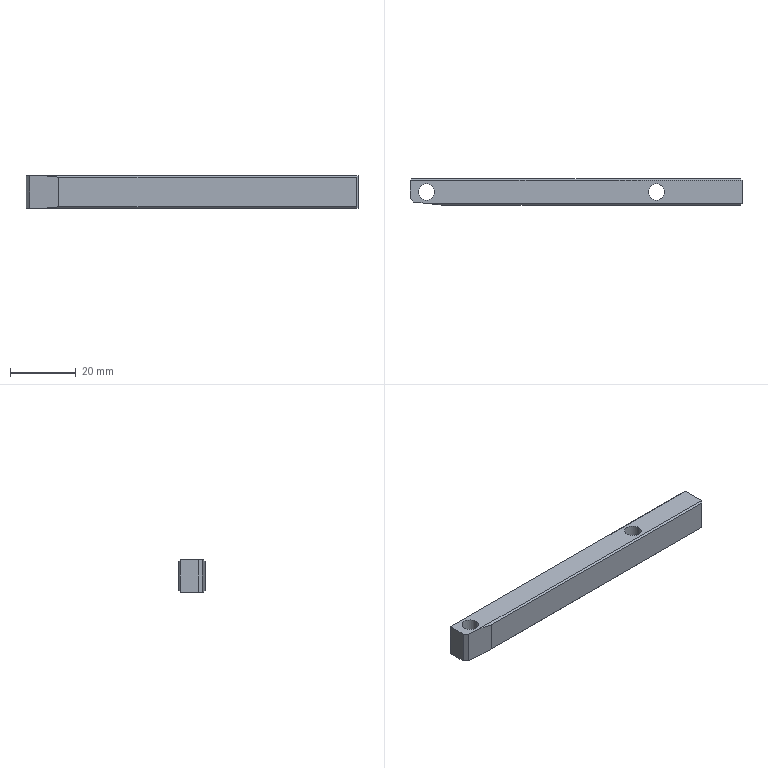Part | SolidWorks | features Chamfer 2, Extrusion 1, HoleWzd 1, ICE 1 | 1 solid | 21 faces | box 101 x 8 x 10 mm | volume 7248 mm3 | plane 15 | cylinder 6 | commonest cylinder face diameters 5 x4 4.2 x2
STEP:
#1=CARTESIAN_POINT('',(27.,0.,2.1));
#2=VERTEX_POINT('',#1);
#3=CARTESIAN_POINT('',(27.,0.,-2.1));
#4=VERTEX_POINT('',#3);
#5=CARTESIAN_POINT('',(27.,0.,2.1));
#6=CARTESIAN_POINT('',(27.,-0.1478,2.1));
#7=CARTESIAN_POINT('',(26.987,-0.2944,2.084));
#8=CARTESIAN_POINT('',(26.937,-0.5774,2.024));
#9=CARTESIAN_POINT('',(26.899,-0.7152,1.979));
#10=CARTESIAN_POINT('',(26.808,-0.9708,1.867));
#11=CARTESIAN_POINT('',(26.753,-1.091,1.799));
#12=CARTESIAN_POINT('',(26.632,-1.311,1.646));
#13=CARTESIAN_POINT('',(26.567,-1.411,1.561));
#14=CARTESIAN_POINT('',(26.431,-1.592,1.376));
#15=CARTESIAN_POINT('',(26.359,-1.674,1.274));
#16=CARTESIAN_POINT('',(26.22,-1.817,1.06));
#17=CARTESIAN_POINT('',(26.151,-1.879,0.9468));
#18=CARTESIAN_POINT('',(26.024,-1.983,0.703));
#19=CARTESIAN_POINT('',(25.966,-2.026,0.5719));
#20=CARTESIAN_POINT('',(25.882,-2.084,0.2961));
#21=CARTESIAN_POINT('',(25.857,-2.1,0.1485));
#22=CARTESIAN_POINT('',(25.856,-2.1,-0.1436));
#23=CARTESIAN_POINT('',(25.881,-2.084,-0.2919));
#24=CARTESIAN_POINT('',(25.965,-2.026,-0.5686));
#25=CARTESIAN_POINT('',(26.023,-1.984,-0.6998));
#26=CARTESIAN_POINT('',(26.212,-1.829,-1.065));
#27=CARTESIAN_POINT('',(26.361,-1.684,-1.281));
#28=CARTESIAN_POINT('',(26.566,-1.412,-1.559));
#29=CARTESIAN_POINT('',(26.632,-1.311,-1.646));
#30=CARTESIAN_POINT('',(26.753,-1.091,-1.799));
#31=CARTESIAN_POINT('',(26.807,-0.9728,-1.866));
#32=CARTESIAN_POINT('',(26.945,-0.5883,-2.035));
#33=CARTESIAN_POINT('',(27.,-0.2971,-2.1));
#34=CARTESIAN_POINT('',(27.,0.,-2.1));
#35=B_SPLINE_CURVE_WITH_KNOTS('',3,(#5,#6,#7,#8,#9,#10,#11,#12,#13,#14,#15,#16,#17,#18,#19,#20,#21,#22,#23,#24,#25,#26,#27,#28,#29,#30,#31,#32,#33,#34),.UNSPECIFIED.,.F.,.F.,(4,2,2,2,2,2,2,2,2,2,2,2,2,2,4),(0.007025,0.007463,0.007902,0.00834,0.008778,0.009216,0.009655,0.01009,0.01053,0.01097,0.01141,0.01228,0.01272,0.01316,0.01404),.UNSPECIFIED.);
#36=EDGE_CURVE('',#2,#4,#35,.T.);
#37=ORIENTED_EDGE('',*,*,#36,.F.);
#38=CARTESIAN_POINT('',(50.5,0.,2.1));
#39=VERTEX_POINT('',#38);
#40=CARTESIAN_POINT('',(50.5,0.,2.1));
#41=DIRECTION('',(1.,0.,0.));
#42=VECTOR('',#41,1000.);
#43=LINE('',#40,#42);
#44=EDGE_CURVE('',#2,#39,#43,.T.);
#45=ORIENTED_EDGE('',*,*,#44,.T.);
#46=CARTESIAN_POINT('',(50.5,0.,-2.1));
#47=VERTEX_POINT('',#46);
#48=CARTESIAN_POINT('',(50.5,0.,0.));
#49=DIRECTION('',(1.,0.,0.));
#50=DIRECTION('',(0.,0.,-1.));
#51=AXIS2_PLACEMENT_3D('',#48,#49,#50);
#52=CIRCLE('',#51,2.1);
#53=EDGE_CURVE('',#39,#47,#52,.T.);
#54=ORIENTED_EDGE('',*,*,#53,.T.);
#55=CARTESIAN_POINT('',(50.5,0.,-2.1));
#56=DIRECTION('',(1.,0.,0.));
#57=VECTOR('',#56,1000.);
#58=LINE('',#55,#57);
#59=EDGE_CURVE('',#4,#47,#58,.T.);
#60=ORIENTED_EDGE('',*,*,#59,.F.);
#61=EDGE_LOOP('',(#37,#45,#54,#60));
#62=FACE_OUTER_BOUND('',#61,.T.);
#63=CARTESIAN_POINT('',(50.5,0.,0.));
#64=DIRECTION('',(1.,0.,0.));
#65=DIRECTION('',(0.,0.,-1.));
#66=AXIS2_PLACEMENT_3D('',#63,#64,#65);
#67=CYLINDRICAL_SURFACE('',#66,2.1);
#68=ADVANCED_FACE('',(#62),#67,.F.);
#69=CARTESIAN_POINT('',(22.,0.,-5.));
#70=VERTEX_POINT('',#69);
#71=CARTESIAN_POINT('',(27.,0.,-5.));
#72=VERTEX_POINT('',#71);
#73=CARTESIAN_POINT('',(24.5,0.,-5.));
#74=DIRECTION('',(0.,0.,1.));
#75=DIRECTION('',(1.,0.,0.));
#76=AXIS2_PLACEMENT_3D('',#73,#74,#75);
#77=CIRCLE('',#76,2.5);
#78=EDGE_CURVE('',#70,#72,#77,.T.);
#79=ORIENTED_EDGE('',*,*,#78,.F.);
#80=CARTESIAN_POINT('',(22.,0.,5.));
#81=VERTEX_POINT('',#80);
#82=CARTESIAN_POINT('',(22.,0.,-5.));
#83=DIRECTION('',(0.,0.,1.));
#84=VECTOR('',#83,1000.);
#85=LINE('',#82,#84);
#86=EDGE_CURVE('',#70,#81,#85,.T.);
#87=ORIENTED_EDGE('',*,*,#86,.T.);
#88=CARTESIAN_POINT('',(27.,0.,5.));
#89=VERTEX_POINT('',#88);
#90=CARTESIAN_POINT('',(24.5,0.,5.));
#91=DIRECTION('',(0.,0.,1.));
#92=DIRECTION('',(1.,0.,0.));
#93=AXIS2_PLACEMENT_3D('',#90,#91,#92);
#94=CIRCLE('',#93,2.5);
#95=EDGE_CURVE('',#81,#89,#94,.T.);
#96=ORIENTED_EDGE('',*,*,#95,.T.);
#97=CARTESIAN_POINT('',(27.,0.,-5.));
#98=DIRECTION('',(0.,0.,1.));
#99=VECTOR('',#98,1000.);
#100=LINE('',#97,#99);
#101=EDGE_CURVE('',#2,#89,#100,.T.);
#102=ORIENTED_EDGE('',*,*,#101,.F.);
#103=ORIENTED_EDGE('',*,*,#36,.T.);
#104=CARTESIAN_POINT('',(27.,0.,-5.));
#105=DIRECTION('',(0.,0.,1.));
#106=VECTOR('',#105,1000.);
#107=LINE('',#104,#106);
#108=EDGE_CURVE('',#72,#4,#107,.T.);
#109=ORIENTED_EDGE('',*,*,#108,.F.);
#110=EDGE_LOOP('',(#79,#87,#96,#102,#103,#109));
#111=FACE_OUTER_BOUND('',#110,.T.);
#112=CARTESIAN_POINT('',(24.5,0.,-5.));
#113=DIRECTION('',(0.,0.,1.));
#114=DIRECTION('',(1.,0.,0.));
#115=AXIS2_PLACEMENT_3D('',#112,#113,#114);
#116=CYLINDRICAL_SURFACE('',#115,2.5);
#117=ADVANCED_FACE('',(#111),#116,.F.);
#118=CARTESIAN_POINT('',(-48.,0.,-5.));
#119=VERTEX_POINT('',#118);
#120=CARTESIAN_POINT('',(-43.,0.,-5.));
#121=VERTEX_POINT('',#120);
#122=CARTESIAN_POINT('',(-45.5,0.,-5.));
#123=DIRECTION('',(0.,0.,1.));
#124=DIRECTION('',(1.,0.,0.));
#125=AXIS2_PLACEMENT_3D('',#122,#123,#124);
#126=CIRCLE('',#125,2.5);
#127=EDGE_CURVE('',#119,#121,#126,.T.);
#128=ORIENTED_EDGE('',*,*,#127,.F.);
#129=CARTESIAN_POINT('',(-48.,0.,5.));
#130=VERTEX_POINT('',#129);
#131=CARTESIAN_POINT('',(-48.,0.,-5.));
#132=DIRECTION('',(0.,0.,1.));
#133=VECTOR('',#132,1000.);
#134=LINE('',#131,#133);
#135=EDGE_CURVE('',#119,#130,#134,.T.);
#136=ORIENTED_EDGE('',*,*,#135,.T.);
#137=CARTESIAN_POINT('',(-43.,0.,5.));
#138=VERTEX_POINT('',#137);
#139=CARTESIAN_POINT('',(-45.5,0.,5.));
#140=DIRECTION('',(0.,0.,1.));
#141=DIRECTION('',(1.,0.,0.));
#142=AXIS2_PLACEMENT_3D('',#139,#140,#141);
#143=CIRCLE('',#142,2.5);
#144=EDGE_CURVE('',#130,#138,#143,.T.);
#145=ORIENTED_EDGE('',*,*,#144,.T.);
#146=CARTESIAN_POINT('',(-43.,0.,-5.));
#147=DIRECTION('',(0.,0.,1.));
#148=VECTOR('',#147,1000.);
#149=LINE('',#146,#148);
#150=EDGE_CURVE('',#121,#138,#149,.T.);
#151=ORIENTED_EDGE('',*,*,#150,.F.);
#152=EDGE_LOOP('',(#128,#136,#145,#151));
#153=FACE_OUTER_BOUND('',#152,.T.);
#154=CARTESIAN_POINT('',(-45.5,0.,-5.));
#155=DIRECTION('',(0.,0.,1.));
#156=DIRECTION('',(1.,0.,0.));
#157=AXIS2_PLACEMENT_3D('',#154,#155,#156);
#158=CYLINDRICAL_SURFACE('',#157,2.5);
#159=ADVANCED_FACE('',(#153),#158,.F.);
#160=CARTESIAN_POINT('',(50.5,0.,0.));
#161=DIRECTION('',(1.,0.,0.));
#162=DIRECTION('',(0.,0.,-1.));
#163=AXIS2_PLACEMENT_3D('',#160,#161,#162);
#164=CIRCLE('',#163,2.1);
#165=EDGE_CURVE('',#47,#39,#164,.T.);
#166=ORIENTED_EDGE('',*,*,#165,.F.);
#167=ORIENTED_EDGE('',*,*,#53,.F.);
#168=EDGE_LOOP('',(#166,#167));
#169=FACE_BOUND('',#168,.T.);
#170=CARTESIAN_POINT('',(50.5,-3.5,-5.));
#171=VERTEX_POINT('',#170);
#172=CARTESIAN_POINT('',(50.5,3.5,-5.));
#173=VERTEX_POINT('',#172);
#174=CARTESIAN_POINT('',(50.5,4.,-5.));
#175=DIRECTION('',(0.,1.,0.));
#176=VECTOR('',#175,1000.);
#177=LINE('',#174,#176);
#178=EDGE_CURVE('',#171,#173,#177,.T.);
#179=ORIENTED_EDGE('',*,*,#178,.T.);
#180=CARTESIAN_POINT('',(50.5,3.5,5.));
#181=VERTEX_POINT('',#180);
#182=CARTESIAN_POINT('',(50.5,3.5,5.));
#183=DIRECTION('',(0.,0.,1.));
#184=VECTOR('',#183,1000.);
#185=LINE('',#182,#184);
#186=EDGE_CURVE('',#173,#181,#185,.T.);
#187=ORIENTED_EDGE('',*,*,#186,.T.);
#188=CARTESIAN_POINT('',(50.5,-3.5,5.));
#189=VERTEX_POINT('',#188);
#190=CARTESIAN_POINT('',(50.5,4.,5.));
#191=DIRECTION('',(0.,1.,0.));
#192=VECTOR('',#191,1000.);
#193=LINE('',#190,#192);
#194=EDGE_CURVE('',#189,#181,#193,.T.);
#195=ORIENTED_EDGE('',*,*,#194,.F.);
#196=CARTESIAN_POINT('',(50.5,-3.5,5.));
#197=DIRECTION('',(0.,0.,-1.));
#198=VECTOR('',#197,1000.);
#199=LINE('',#196,#198);
#200=EDGE_CURVE('',#189,#171,#199,.T.);
#201=ORIENTED_EDGE('',*,*,#200,.T.);
#202=EDGE_LOOP('',(#179,#187,#195,#201));
#203=FACE_OUTER_BOUND('',#202,.T.);
#204=CARTESIAN_POINT('',(50.5,4.,5.));
#205=DIRECTION('',(-1.,0.,0.));
#206=DIRECTION('',(0.,-1.,0.));
#207=AXIS2_PLACEMENT_3D('',#204,#205,#206);
#208=PLANE('',#207);
#209=ADVANCED_FACE('',(#169,#203),#208,.F.);
#210=CARTESIAN_POINT('',(50.,4.,4.5));
#211=VERTEX_POINT('',#210);
#212=CARTESIAN_POINT('',(50.,4.,-4.5));
#213=VERTEX_POINT('',#212);
#214=CARTESIAN_POINT('',(50.,4.,5.));
#215=DIRECTION('',(0.,0.,-1.));
#216=VECTOR('',#215,1000.);
#217=LINE('',#214,#216);
#218=EDGE_CURVE('',#211,#213,#217,.T.);
#219=ORIENTED_EDGE('',*,*,#218,.T.);
#220=CARTESIAN_POINT('',(-50.,4.,-4.5));
#221=VERTEX_POINT('',#220);
#222=CARTESIAN_POINT('',(-50.5,4.,-4.5));
#223=DIRECTION('',(-1.,0.,0.));
#224=VECTOR('',#223,1000.);
#225=LINE('',#222,#224);
#226=EDGE_CURVE('',#213,#221,#225,.T.);
#227=ORIENTED_EDGE('',*,*,#226,.T.);
#228=CARTESIAN_POINT('',(-50.,4.,4.5));
#229=VERTEX_POINT('',#228);
#230=CARTESIAN_POINT('',(-50.,4.,5.));
#231=DIRECTION('',(0.,0.,1.));
#232=VECTOR('',#231,1000.);
#233=LINE('',#230,#232);
#234=EDGE_CURVE('',#221,#229,#233,.T.);
#235=ORIENTED_EDGE('',*,*,#234,.T.);
#236=CARTESIAN_POINT('',(50.5,4.,4.5));
#237=DIRECTION('',(1.,0.,0.));
#238=VECTOR('',#237,1000.);
#239=LINE('',#236,#238);
#240=EDGE_CURVE('',#229,#211,#239,.T.);
#241=ORIENTED_EDGE('',*,*,#240,.T.);
#242=EDGE_LOOP('',(#219,#227,#235,#241));
#243=FACE_OUTER_BOUND('',#242,.T.);
#244=CARTESIAN_POINT('',(-50.5,4.,5.));
#245=DIRECTION('',(0.,-1.,0.));
#246=DIRECTION('',(0.,0.,-1.));
#247=AXIS2_PLACEMENT_3D('',#244,#245,#246);
#248=PLANE('',#247);
#249=ADVANCED_FACE('',(#243),#248,.F.);
#250=CARTESIAN_POINT('',(-50.5,3.5,-5.));
#251=VERTEX_POINT('',#250);
#252=CARTESIAN_POINT('',(-50.5,-1.949,-5.));
#253=VERTEX_POINT('',#252);
#254=CARTESIAN_POINT('',(-50.5,4.,-5.));
#255=DIRECTION('',(0.,-1.,0.));
#256=VECTOR('',#255,1000.);
#257=LINE('',#254,#256);
#258=EDGE_CURVE('',#251,#253,#257,.T.);
#259=ORIENTED_EDGE('',*,*,#258,.T.);
#260=CARTESIAN_POINT('',(-50.5,-1.949,5.));
#261=VERTEX_POINT('',#260);
#262=CARTESIAN_POINT('',(-50.5,-1.949,5.));
#263=DIRECTION('',(0.,0.,1.));
#264=VECTOR('',#263,1000.);
#265=LINE('',#262,#264);
#266=EDGE_CURVE('',#253,#261,#265,.T.);
#267=ORIENTED_EDGE('',*,*,#266,.T.);
#268=CARTESIAN_POINT('',(-50.5,3.5,5.));
#269=VERTEX_POINT('',#268);
#270=CARTESIAN_POINT('',(-50.5,4.,5.));
#271=DIRECTION('',(0.,-1.,0.));
#272=VECTOR('',#271,1000.);
#273=LINE('',#270,#272);
#274=EDGE_CURVE('',#269,#261,#273,.T.);
#275=ORIENTED_EDGE('',*,*,#274,.F.);
#276=CARTESIAN_POINT('',(-50.5,3.5,5.));
#277=DIRECTION('',(0.,0.,-1.));
#278=VECTOR('',#277,1000.);
#279=LINE('',#276,#278);
#280=EDGE_CURVE('',#269,#251,#279,.T.);
#281=ORIENTED_EDGE('',*,*,#280,.T.);
#282=EDGE_LOOP('',(#259,#267,#275,#281));
#283=FACE_OUTER_BOUND('',#282,.T.);
#284=CARTESIAN_POINT('',(-50.5,4.,5.));
#285=DIRECTION('',(1.,0.,0.));
#286=DIRECTION('',(0.,0.,-1.));
#287=AXIS2_PLACEMENT_3D('',#284,#285,#286);
#288=PLANE('',#287);
#289=ADVANCED_FACE('',(#283),#288,.F.);
#290=CARTESIAN_POINT('',(-49.383,-3.066,5.));
#291=VERTEX_POINT('',#290);
#292=CARTESIAN_POINT('',(-45.257,-3.5,5.));
#293=VERTEX_POINT('',#292);
#294=CARTESIAN_POINT('',(-40.5,-4.,5.));
#295=DIRECTION('',(0.9945,-0.1045,0.));
#296=VECTOR('',#295,1000.);
#297=LINE('',#294,#296);
#298=EDGE_CURVE('',#291,#293,#297,.T.);
#299=ORIENTED_EDGE('',*,*,#298,.F.);
#300=CARTESIAN_POINT('',(-49.383,-3.066,-5.));
#301=VERTEX_POINT('',#300);
#302=CARTESIAN_POINT('',(-49.383,-3.066,5.));
#303=DIRECTION('',(0.,0.,-1.));
#304=VECTOR('',#303,1000.);
#305=LINE('',#302,#304);
#306=EDGE_CURVE('',#291,#301,#305,.T.);
#307=ORIENTED_EDGE('',*,*,#306,.T.);
#308=CARTESIAN_POINT('',(-45.257,-3.5,-5.));
#309=VERTEX_POINT('',#308);
#310=CARTESIAN_POINT('',(-40.5,-4.,-5.));
#311=DIRECTION('',(0.9945,-0.1045,0.));
#312=VECTOR('',#311,1000.);
#313=LINE('',#310,#312);
#314=EDGE_CURVE('',#301,#309,#313,.T.);
#315=ORIENTED_EDGE('',*,*,#314,.T.);
#316=CARTESIAN_POINT('',(-40.5,-4.,-4.5));
#317=VERTEX_POINT('',#316);
#318=CARTESIAN_POINT('',(-40.5,-4.,-4.5));
#319=DIRECTION('',(0.9891,-0.104,0.104));
#320=VECTOR('',#319,1000.);
#321=LINE('',#318,#320);
#322=EDGE_CURVE('',#309,#317,#321,.T.);
#323=ORIENTED_EDGE('',*,*,#322,.T.);
#324=CARTESIAN_POINT('',(-40.5,-4.,4.5));
#325=VERTEX_POINT('',#324);
#326=CARTESIAN_POINT('',(-40.5,-4.,5.));
#327=DIRECTION('',(0.,0.,-1.));
#328=VECTOR('',#327,1000.);
#329=LINE('',#326,#328);
#330=EDGE_CURVE('',#325,#317,#329,.T.);
#331=ORIENTED_EDGE('',*,*,#330,.F.);
#332=CARTESIAN_POINT('',(-0.9783,-8.154,0.3461));
#333=DIRECTION('',(-0.9891,0.104,0.104));
#334=VECTOR('',#333,1000.);
#335=LINE('',#332,#334);
#336=EDGE_CURVE('',#325,#293,#335,.T.);
#337=ORIENTED_EDGE('',*,*,#336,.T.);
#338=EDGE_LOOP('',(#299,#307,#315,#323,#331,#337));
#339=FACE_OUTER_BOUND('',#338,.T.);
#340=CARTESIAN_POINT('',(-40.5,-4.,5.));
#341=DIRECTION('',(0.1045,0.9945,0.));
#342=DIRECTION('',(-0.9945,0.1045,0.));
#343=AXIS2_PLACEMENT_3D('',#340,#341,#342);
#344=PLANE('',#343);
#345=ADVANCED_FACE('',(#339),#344,.F.);
#346=ORIENTED_EDGE('',*,*,#330,.T.);
#347=CARTESIAN_POINT('',(50.,-4.,-4.5));
#348=VERTEX_POINT('',#347);
#349=CARTESIAN_POINT('',(-40.5,-4.,-4.5));
#350=DIRECTION('',(1.,0.,0.));
#351=VECTOR('',#350,1000.);
#352=LINE('',#349,#351);
#353=EDGE_CURVE('',#317,#348,#352,.T.);
#354=ORIENTED_EDGE('',*,*,#353,.T.);
#355=CARTESIAN_POINT('',(50.,-4.,4.5));
#356=VERTEX_POINT('',#355);
#357=CARTESIAN_POINT('',(50.,-4.,5.));
#358=DIRECTION('',(0.,0.,1.));
#359=VECTOR('',#358,1000.);
#360=LINE('',#357,#359);
#361=EDGE_CURVE('',#348,#356,#360,.T.);
#362=ORIENTED_EDGE('',*,*,#361,.T.);
#363=CARTESIAN_POINT('',(-40.5,-4.,4.5));
#364=DIRECTION('',(-1.,0.,0.));
#365=VECTOR('',#364,1000.);
#366=LINE('',#363,#365);
#367=EDGE_CURVE('',#356,#325,#366,.T.);
#368=ORIENTED_EDGE('',*,*,#367,.T.);
#369=EDGE_LOOP('',(#346,#354,#362,#368));
#370=FACE_OUTER_BOUND('',#369,.T.);
#371=CARTESIAN_POINT('',(-40.5,-4.,5.));
#372=DIRECTION('',(0.,1.,0.));
#373=DIRECTION('',(-1.,0.,0.));
#374=AXIS2_PLACEMENT_3D('',#371,#372,#373);
#375=PLANE('',#374);
#376=ADVANCED_FACE('',(#370),#375,.F.);
#377=CARTESIAN_POINT('',(24.5,0.,5.));
#378=DIRECTION('',(0.,0.,1.));
#379=DIRECTION('',(1.,0.,0.));
#380=AXIS2_PLACEMENT_3D('',#377,#378,#379);
#381=CIRCLE('',#380,2.5);
#382=EDGE_CURVE('',#89,#81,#381,.T.);
#383=ORIENTED_EDGE('',*,*,#382,.F.);
#384=ORIENTED_EDGE('',*,*,#95,.F.);
#385=EDGE_LOOP('',(#383,#384));
#386=FACE_BOUND('',#385,.T.);
#387=CARTESIAN_POINT('',(-45.5,0.,5.));
#388=DIRECTION('',(0.,0.,1.));
#389=DIRECTION('',(1.,0.,0.));
#390=AXIS2_PLACEMENT_3D('',#387,#388,#389);
#391=CIRCLE('',#390,2.5);
#392=EDGE_CURVE('',#138,#130,#391,.T.);
#393=ORIENTED_EDGE('',*,*,#392,.F.);
#394=ORIENTED_EDGE('',*,*,#144,.F.);
#395=EDGE_LOOP('',(#393,#394));
#396=FACE_BOUND('',#395,.T.);
#397=ORIENTED_EDGE('',*,*,#274,.T.);
#398=CARTESIAN_POINT('',(-26.224,-26.224,5.));
#399=DIRECTION('',(0.7071,-0.7071,0.));
#400=VECTOR('',#399,1000.);
#401=LINE('',#398,#400);
#402=EDGE_CURVE('',#261,#291,#401,.T.);
#403=ORIENTED_EDGE('',*,*,#402,.T.);
#404=ORIENTED_EDGE('',*,*,#298,.T.);
#405=CARTESIAN_POINT('',(50.5,-3.5,5.));
#406=DIRECTION('',(1.,0.,0.));
#407=VECTOR('',#406,1000.);
#408=LINE('',#405,#407);
#409=EDGE_CURVE('',#293,#189,#408,.T.);
#410=ORIENTED_EDGE('',*,*,#409,.T.);
#411=ORIENTED_EDGE('',*,*,#194,.T.);
#412=CARTESIAN_POINT('',(-50.5,3.5,5.));
#413=DIRECTION('',(-1.,0.,0.));
#414=VECTOR('',#413,1000.);
#415=LINE('',#412,#414);
#416=EDGE_CURVE('',#181,#269,#415,.T.);
#417=ORIENTED_EDGE('',*,*,#416,.T.);
#418=EDGE_LOOP('',(#397,#403,#404,#410,#411,#417));
#419=FACE_OUTER_BOUND('',#418,.T.);
#420=CARTESIAN_POINT('',(0.,0.,5.));
#421=DIRECTION('',(0.,0.,1.));
#422=DIRECTION('',(1.,0.,0.));
#423=AXIS2_PLACEMENT_3D('',#420,#421,#422);
#424=PLANE('',#423);
#425=ADVANCED_FACE('',(#386,#396,#419),#424,.T.);
#426=CARTESIAN_POINT('',(24.5,0.,-5.));
#427=DIRECTION('',(0.,0.,1.));
#428=DIRECTION('',(1.,0.,0.));
#429=AXIS2_PLACEMENT_3D('',#426,#427,#428);
#430=CIRCLE('',#429,2.5);
#431=EDGE_CURVE('',#72,#70,#430,.T.);
#432=ORIENTED_EDGE('',*,*,#431,.T.);
#433=ORIENTED_EDGE('',*,*,#78,.T.);
#434=EDGE_LOOP('',(#432,#433));
#435=FACE_BOUND('',#434,.T.);
#436=CARTESIAN_POINT('',(-45.5,0.,-5.));
#437=DIRECTION('',(0.,0.,1.));
#438=DIRECTION('',(1.,0.,0.));
#439=AXIS2_PLACEMENT_3D('',#436,#437,#438);
#440=CIRCLE('',#439,2.5);
#441=EDGE_CURVE('',#121,#119,#440,.T.);
#442=ORIENTED_EDGE('',*,*,#441,.T.);
#443=ORIENTED_EDGE('',*,*,#127,.T.);
#444=EDGE_LOOP('',(#442,#443));
#445=FACE_BOUND('',#444,.T.);
#446=ORIENTED_EDGE('',*,*,#314,.F.);
#447=CARTESIAN_POINT('',(-49.383,-3.066,-5.));
#448=DIRECTION('',(-0.7071,0.7071,0.));
#449=VECTOR('',#448,1000.);
#450=LINE('',#447,#449);
#451=EDGE_CURVE('',#301,#253,#450,.T.);
#452=ORIENTED_EDGE('',*,*,#451,.T.);
#453=ORIENTED_EDGE('',*,*,#258,.F.);
#454=CARTESIAN_POINT('',(0.,3.5,-5.));
#455=DIRECTION('',(1.,0.,0.));
#456=VECTOR('',#455,1000.);
#457=LINE('',#454,#456);
#458=EDGE_CURVE('',#251,#173,#457,.T.);
#459=ORIENTED_EDGE('',*,*,#458,.T.);
#460=ORIENTED_EDGE('',*,*,#178,.F.);
#461=CARTESIAN_POINT('',(0.,-3.5,-5.));
#462=DIRECTION('',(-1.,0.,0.));
#463=VECTOR('',#462,1000.);
#464=LINE('',#461,#463);
#465=EDGE_CURVE('',#171,#309,#464,.T.);
#466=ORIENTED_EDGE('',*,*,#465,.T.);
#467=EDGE_LOOP('',(#446,#452,#453,#459,#460,#466));
#468=FACE_OUTER_BOUND('',#467,.T.);
#469=CARTESIAN_POINT('',(0.,0.,-5.));
#470=DIRECTION('',(0.,0.,1.));
#471=DIRECTION('',(1.,0.,0.));
#472=AXIS2_PLACEMENT_3D('',#469,#470,#471);
#473=PLANE('',#472);
#474=ADVANCED_FACE('',(#435,#445,#468),#473,.F.);
#475=ORIENTED_EDGE('',*,*,#135,.F.);
#476=ORIENTED_EDGE('',*,*,#441,.F.);
#477=ORIENTED_EDGE('',*,*,#150,.T.);
#478=ORIENTED_EDGE('',*,*,#392,.T.);
#479=EDGE_LOOP('',(#475,#476,#477,#478));
#480=FACE_OUTER_BOUND('',#479,.T.);
#481=CARTESIAN_POINT('',(-45.5,0.,-5.));
#482=DIRECTION('',(0.,0.,1.));
#483=DIRECTION('',(1.,0.,0.));
#484=AXIS2_PLACEMENT_3D('',#481,#482,#483);
#485=CYLINDRICAL_SURFACE('',#484,2.5);
#486=ADVANCED_FACE('',(#480),#485,.F.);
#487=ORIENTED_EDGE('',*,*,#86,.F.);
#488=ORIENTED_EDGE('',*,*,#431,.F.);
#489=ORIENTED_EDGE('',*,*,#108,.T.);
#490=CARTESIAN_POINT('',(27.,0.,-2.1));
#491=CARTESIAN_POINT('',(27.,0.1488,-2.1));
#492=CARTESIAN_POINT('',(26.987,0.2939,-2.084));
#493=CARTESIAN_POINT('',(26.937,0.5771,-2.024));
#494=CARTESIAN_POINT('',(26.899,0.7152,-1.979));
#495=CARTESIAN_POINT('',(26.808,0.9708,-1.867));
#496=CARTESIAN_POINT('',(26.753,1.092,-1.799));
#497=CARTESIAN_POINT('',(26.632,1.312,-1.645));
#498=CARTESIAN_POINT('',(26.567,1.411,-1.56));
#499=CARTESIAN_POINT('',(26.43,1.593,-1.375));
#500=CARTESIAN_POINT('',(26.359,1.675,-1.273));
#501=CARTESIAN_POINT('',(26.219,1.818,-1.059));
#502=CARTESIAN_POINT('',(26.15,1.88,-0.9451));
#503=CARTESIAN_POINT('',(26.023,1.984,-0.7013));
#504=CARTESIAN_POINT('',(25.965,2.026,-0.5697));
#505=CARTESIAN_POINT('',(25.882,2.084,-0.2934));
#506=CARTESIAN_POINT('',(25.856,2.1,-0.1452));
#507=CARTESIAN_POINT('',(25.857,2.1,0.1475));
#508=CARTESIAN_POINT('',(25.882,2.084,0.2959));
#509=CARTESIAN_POINT('',(25.966,2.026,0.5714));
#510=CARTESIAN_POINT('',(26.024,1.983,0.7029));
#511=CARTESIAN_POINT('',(26.151,1.879,0.9466));
#512=CARTESIAN_POINT('',(26.22,1.817,1.06));
#513=CARTESIAN_POINT('',(26.36,1.674,1.275));
#514=CARTESIAN_POINT('',(26.431,1.591,1.376));
#515=CARTESIAN_POINT('',(26.568,1.41,1.562));
#516=CARTESIAN_POINT('',(26.633,1.31,1.647));
#517=CARTESIAN_POINT('',(26.754,1.09,1.8));
#518=CARTESIAN_POINT('',(26.808,0.9691,1.868));
#519=CARTESIAN_POINT('',(26.9,0.7139,1.98));
#520=CARTESIAN_POINT('',(26.937,0.5757,2.025));
#521=CARTESIAN_POINT('',(26.987,0.2927,2.085));
#522=CARTESIAN_POINT('',(27.,0.148,2.1));
#523=CARTESIAN_POINT('',(27.,0.,2.1));
#524=B_SPLINE_CURVE_WITH_KNOTS('',3,(#490,#491,#492,#493,#494,#495,#496,#497,#498,#499,#500,#501,#502,#503,#504,#505,#506,#507,#508,#509,#510,#511,#512,#513,#514,#515,#516,#517,#518,#519,#520,#521,#522,#523),.UNSPECIFIED.,.F.,.F.,(4,2,2,2,2,2,2,2,2,2,2,2,2,2,2,2,4),(0.,0.0004391,0.0008781,0.001317,0.001756,0.002195,0.002634,0.003074,0.003513,0.003952,0.004391,0.00483,0.005269,0.005708,0.006147,0.006586,0.007025),.UNSPECIFIED.);
#525=EDGE_CURVE('',#4,#2,#524,.T.);
#526=ORIENTED_EDGE('',*,*,#525,.T.);
#527=ORIENTED_EDGE('',*,*,#101,.T.);
#528=ORIENTED_EDGE('',*,*,#382,.T.);
#529=EDGE_LOOP('',(#487,#488,#489,#526,#527,#528));
#530=FACE_OUTER_BOUND('',#529,.T.);
#531=CARTESIAN_POINT('',(24.5,0.,-5.));
#532=DIRECTION('',(0.,0.,1.));
#533=DIRECTION('',(1.,0.,0.));
#534=AXIS2_PLACEMENT_3D('',#531,#532,#533);
#535=CYLINDRICAL_SURFACE('',#534,2.5);
#536=ADVANCED_FACE('',(#530),#535,.F.);
#537=CARTESIAN_POINT('',(-33.667,20.333,-11.833));
#538=DIRECTION('',(0.5774,0.5774,-0.5774));
#539=VECTOR('',#538,1000.);
#540=LINE('',#537,#539);
#541=EDGE_CURVE('',#269,#229,#540,.T.);
#542=ORIENTED_EDGE('',*,*,#541,.F.);
#543=ORIENTED_EDGE('',*,*,#416,.F.);
#544=CARTESIAN_POINT('',(50.167,3.833,4.667));
#545=DIRECTION('',(0.5774,-0.5774,0.5774));
#546=VECTOR('',#545,1000.);
#547=LINE('',#544,#546);
#548=EDGE_CURVE('',#211,#181,#547,.T.);
#549=ORIENTED_EDGE('',*,*,#548,.F.);
#550=ORIENTED_EDGE('',*,*,#240,.F.);
#551=EDGE_LOOP('',(#542,#543,#549,#550));
#552=FACE_OUTER_BOUND('',#551,.T.);
#553=CARTESIAN_POINT('',(0.,3.5,5.));
#554=DIRECTION('',(0.,0.7071,0.7071));
#555=DIRECTION('',(1.,0.,0.));
#556=AXIS2_PLACEMENT_3D('',#553,#554,#555);
#557=PLANE('',#556);
#558=ADVANCED_FACE('',(#552),#557,.T.);
#559=ORIENTED_EDGE('',*,*,#548,.T.);
#560=ORIENTED_EDGE('',*,*,#186,.F.);
#561=CARTESIAN_POINT('',(46.833,7.167,-1.333));
#562=DIRECTION('',(0.5774,-0.5774,-0.5774));
#563=VECTOR('',#562,1000.);
#564=LINE('',#561,#563);
#565=EDGE_CURVE('',#213,#173,#564,.T.);
#566=ORIENTED_EDGE('',*,*,#565,.F.);
#567=ORIENTED_EDGE('',*,*,#218,.F.);
#568=EDGE_LOOP('',(#559,#560,#566,#567));
#569=FACE_OUTER_BOUND('',#568,.T.);
#570=CARTESIAN_POINT('',(50.,4.,5.));
#571=DIRECTION('',(-0.7071,-0.7071,0.));
#572=DIRECTION('',(0.,0.,-1.));
#573=AXIS2_PLACEMENT_3D('',#570,#571,#572);
#574=PLANE('',#573);
#575=ADVANCED_FACE('',(#569),#574,.F.);
#576=ORIENTED_EDGE('',*,*,#541,.T.);
#577=ORIENTED_EDGE('',*,*,#234,.F.);
#578=CARTESIAN_POINT('',(-47.167,6.833,-1.667));
#579=DIRECTION('',(0.5774,0.5774,0.5774));
#580=VECTOR('',#579,1000.);
#581=LINE('',#578,#580);
#582=EDGE_CURVE('',#251,#221,#581,.T.);
#583=ORIENTED_EDGE('',*,*,#582,.F.);
#584=ORIENTED_EDGE('',*,*,#280,.F.);
#585=EDGE_LOOP('',(#576,#577,#583,#584));
#586=FACE_OUTER_BOUND('',#585,.T.);
#587=CARTESIAN_POINT('',(-50.5,3.5,5.));
#588=DIRECTION('',(0.7071,-0.7071,0.));
#589=DIRECTION('',(0.,0.,-1.));
#590=AXIS2_PLACEMENT_3D('',#587,#588,#589);
#591=PLANE('',#590);
#592=ADVANCED_FACE('',(#586),#591,.F.);
#593=ORIENTED_EDGE('',*,*,#565,.T.);
#594=ORIENTED_EDGE('',*,*,#458,.F.);
#595=ORIENTED_EDGE('',*,*,#582,.T.);
#596=ORIENTED_EDGE('',*,*,#226,.F.);
#597=EDGE_LOOP('',(#593,#594,#595,#596));
#598=FACE_OUTER_BOUND('',#597,.T.);
#599=CARTESIAN_POINT('',(-50.5,4.,-4.5));
#600=DIRECTION('',(0.,-0.7071,0.7071));
#601=DIRECTION('',(-1.,0.,0.));
#602=AXIS2_PLACEMENT_3D('',#599,#600,#601);
#603=PLANE('',#602);
#604=ADVANCED_FACE('',(#598),#603,.F.);
#605=ORIENTED_EDGE('',*,*,#336,.F.);
#606=ORIENTED_EDGE('',*,*,#367,.F.);
#607=CARTESIAN_POINT('',(50.5,-3.5,5.));
#608=DIRECTION('',(-0.5774,-0.5774,-0.5774));
#609=VECTOR('',#608,1000.);
#610=LINE('',#607,#609);
#611=EDGE_CURVE('',#189,#356,#610,.T.);
#612=ORIENTED_EDGE('',*,*,#611,.F.);
#613=ORIENTED_EDGE('',*,*,#409,.F.);
#614=EDGE_LOOP('',(#605,#606,#612,#613));
#615=FACE_OUTER_BOUND('',#614,.T.);
#616=CARTESIAN_POINT('',(0.,-3.5,5.));
#617=DIRECTION('',(0.,-0.7071,0.7071));
#618=DIRECTION('',(-1.,0.,0.));
#619=AXIS2_PLACEMENT_3D('',#616,#617,#618);
#620=PLANE('',#619);
#621=ADVANCED_FACE('',(#615),#620,.T.);
#622=ORIENTED_EDGE('',*,*,#611,.T.);
#623=ORIENTED_EDGE('',*,*,#361,.F.);
#624=CARTESIAN_POINT('',(47.167,-6.833,-1.667));
#625=DIRECTION('',(-0.5774,-0.5774,0.5774));
#626=VECTOR('',#625,1000.);
#627=LINE('',#624,#626);
#628=EDGE_CURVE('',#171,#348,#627,.T.);
#629=ORIENTED_EDGE('',*,*,#628,.F.);
#630=ORIENTED_EDGE('',*,*,#200,.F.);
#631=EDGE_LOOP('',(#622,#623,#629,#630));
#632=FACE_OUTER_BOUND('',#631,.T.);
#633=CARTESIAN_POINT('',(50.5,-3.5,5.));
#634=DIRECTION('',(-0.7071,0.7071,0.));
#635=DIRECTION('',(0.,0.,-1.));
#636=AXIS2_PLACEMENT_3D('',#633,#634,#635);
#637=PLANE('',#636);
#638=ADVANCED_FACE('',(#632),#637,.F.);
#639=ORIENTED_EDGE('',*,*,#322,.F.);
#640=ORIENTED_EDGE('',*,*,#465,.F.);
#641=ORIENTED_EDGE('',*,*,#628,.T.);
#642=ORIENTED_EDGE('',*,*,#353,.F.);
#643=EDGE_LOOP('',(#639,#640,#641,#642));
#644=FACE_OUTER_BOUND('',#643,.T.);
#645=CARTESIAN_POINT('',(-40.5,-4.,-4.5));
#646=DIRECTION('',(0.,0.7071,0.7071));
#647=DIRECTION('',(1.,0.,0.));
#648=AXIS2_PLACEMENT_3D('',#645,#646,#647);
#649=PLANE('',#648);
#650=ADVANCED_FACE('',(#644),#649,.F.);
#651=ORIENTED_EDGE('',*,*,#402,.F.);
#652=ORIENTED_EDGE('',*,*,#266,.F.);
#653=ORIENTED_EDGE('',*,*,#451,.F.);
#654=ORIENTED_EDGE('',*,*,#306,.F.);
#655=EDGE_LOOP('',(#651,#652,#653,#654));
#656=FACE_OUTER_BOUND('',#655,.T.);
#657=CARTESIAN_POINT('',(-49.383,-3.066,5.));
#658=DIRECTION('',(0.7071,0.7071,0.));
#659=DIRECTION('',(0.,0.,-1.));
#660=AXIS2_PLACEMENT_3D('',#657,#658,#659);
#661=PLANE('',#660);
#662=ADVANCED_FACE('',(#656),#661,.F.);
#663=ORIENTED_EDGE('',*,*,#44,.F.);
#664=ORIENTED_EDGE('',*,*,#525,.F.);
#665=ORIENTED_EDGE('',*,*,#59,.T.);
#666=ORIENTED_EDGE('',*,*,#165,.T.);
#667=EDGE_LOOP('',(#663,#664,#665,#666));
#668=FACE_OUTER_BOUND('',#667,.T.);
#669=CARTESIAN_POINT('',(50.5,0.,0.));
#670=DIRECTION('',(1.,0.,0.));
#671=DIRECTION('',(0.,0.,-1.));
#672=AXIS2_PLACEMENT_3D('',#669,#670,#671);
#673=CYLINDRICAL_SURFACE('',#672,2.1);
#674=ADVANCED_FACE('',(#668),#673,.F.);
#675=CLOSED_SHELL('',(#68,#117,#159,#209,#249,#289,#345,#376,#425,#474,#486,#536,#558,#575,#592,#604,#621,#638,#650,#662,#674));
#676=MANIFOLD_SOLID_BREP('',#675);
#677=CARTESIAN_POINT('',(0.,0.,0.));
#678=DIRECTION('',(0.,0.,1.));
#679=DIRECTION('',(1.,0.,0.));
#680=AXIS2_PLACEMENT_3D('',#677,#678,#679);
#681=(LENGTH_UNIT()NAMED_UNIT(*)SI_UNIT(.MILLI.,.METRE.));
#682=UNCERTAINTY_MEASURE_WITH_UNIT(LENGTH_MEASURE(0.00001),#681,'','');
#683=(NAMED_UNIT(*)PLANE_ANGLE_UNIT()SI_UNIT($,.RADIAN.));
#684=(NAMED_UNIT(*)SI_UNIT($,.STERADIAN.)SOLID_ANGLE_UNIT());
#685=(GEOMETRIC_REPRESENTATION_CONTEXT(3)GLOBAL_UNCERTAINTY_ASSIGNED_CONTEXT((#682))GLOBAL_UNIT_ASSIGNED_CONTEXT((#681,#683,#684))REPRESENTATION_CONTEXT('',''));
#686=ADVANCED_BREP_SHAPE_REPRESENTATION('',(#676,#680),#685);